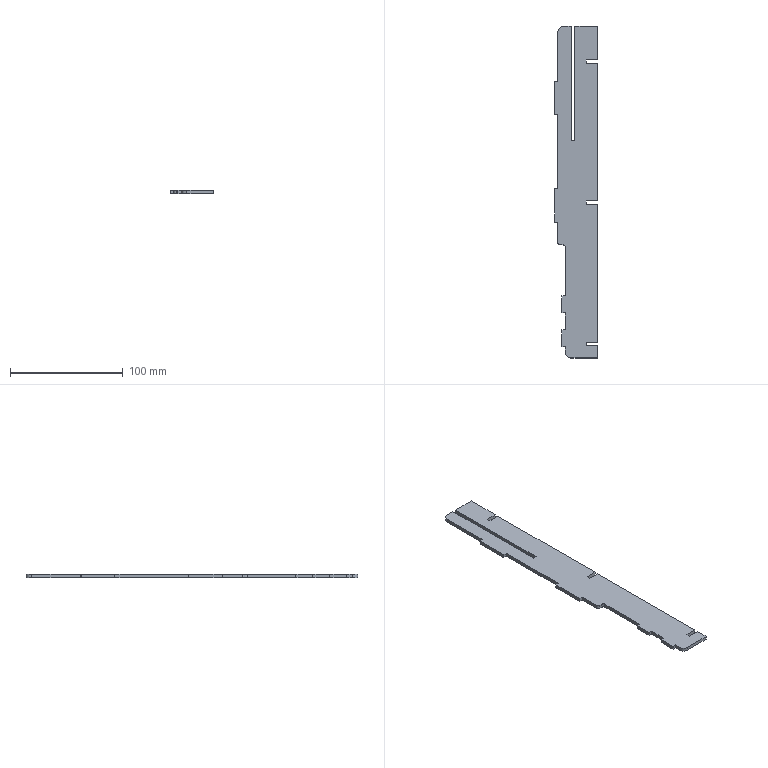Part | SolidWorks | features FlatPattern 1, SMBaseFlange 1, SheetMetal 1 | 1 solid | 46 faces | box 38 x 294.081 x 3.2 mm | volume 30340 mm3 | plane 40 | cylinder 6 | commonest cylinder face diameters 1 x2 4 x2 10 x2
STEP:
#1=CARTESIAN_POINT('',(-378.4,-209.357,0.));
#2=VERTEX_POINT('',#1);
#3=CARTESIAN_POINT('',(-378.4,-198.476,0.));
#4=VERTEX_POINT('',#3);
#5=CARTESIAN_POINT('',(-378.4,-198.476,0.));
#6=DIRECTION('',(-0.000000011,1.,0.));
#7=VECTOR('',#6,1000.);
#8=LINE('',#5,#7);
#9=EDGE_CURVE('',#2,#4,#8,.T.);
#10=ORIENTED_EDGE('',*,*,#9,.F.);
#11=CARTESIAN_POINT('',(-378.4,-209.357,-3.2));
#12=VERTEX_POINT('',#11);
#13=CARTESIAN_POINT('',(-378.4,-209.357,-3.2));
#14=DIRECTION('',(0.,0.,1.));
#15=VECTOR('',#14,1000.);
#16=LINE('',#13,#15);
#17=EDGE_CURVE('',#12,#2,#16,.T.);
#18=ORIENTED_EDGE('',*,*,#17,.F.);
#19=CARTESIAN_POINT('',(-378.4,-198.476,-3.2));
#20=VERTEX_POINT('',#19);
#21=CARTESIAN_POINT('',(-378.4,-198.476,-3.2));
#22=DIRECTION('',(-0.000000011,1.,0.));
#23=VECTOR('',#22,1000.);
#24=LINE('',#21,#23);
#25=EDGE_CURVE('',#12,#20,#24,.T.);
#26=ORIENTED_EDGE('',*,*,#25,.T.);
#27=CARTESIAN_POINT('',(-378.4,-198.476,-3.2));
#28=DIRECTION('',(0.,0.,1.));
#29=VECTOR('',#28,1000.);
#30=LINE('',#27,#29);
#31=EDGE_CURVE('',#20,#4,#30,.T.);
#32=ORIENTED_EDGE('',*,*,#31,.T.);
#33=EDGE_LOOP('',(#10,#18,#26,#32));
#34=FACE_OUTER_BOUND('',#33,.T.);
#35=CARTESIAN_POINT('',(-378.4,-198.476,-3.2));
#36=DIRECTION('',(1.,0.000000011,0.));
#37=DIRECTION('',(-0.000000011,1.,0.));
#38=AXIS2_PLACEMENT_3D('',#35,#36,#37);
#39=PLANE('',#38);
#40=ADVANCED_FACE('',(#34),#39,.T.);
#41=CARTESIAN_POINT('',(-401.9,-209.357,0.));
#42=VERTEX_POINT('',#41);
#43=CARTESIAN_POINT('',(-401.9,-209.357,0.));
#44=DIRECTION('',(1.,0.,0.));
#45=VECTOR('',#44,1000.);
#46=LINE('',#43,#45);
#47=EDGE_CURVE('',#42,#2,#46,.T.);
#48=ORIENTED_EDGE('',*,*,#47,.F.);
#49=CARTESIAN_POINT('',(-401.9,-209.357,-3.2));
#50=VERTEX_POINT('',#49);
#51=CARTESIAN_POINT('',(-401.9,-209.357,-3.2));
#52=DIRECTION('',(0.,0.,1.));
#53=VECTOR('',#52,1000.);
#54=LINE('',#51,#53);
#55=EDGE_CURVE('',#50,#42,#54,.T.);
#56=ORIENTED_EDGE('',*,*,#55,.F.);
#57=CARTESIAN_POINT('',(-401.9,-209.357,-3.2));
#58=DIRECTION('',(1.,0.,0.));
#59=VECTOR('',#58,1000.);
#60=LINE('',#57,#59);
#61=EDGE_CURVE('',#50,#12,#60,.T.);
#62=ORIENTED_EDGE('',*,*,#61,.T.);
#63=ORIENTED_EDGE('',*,*,#17,.T.);
#64=EDGE_LOOP('',(#48,#56,#62,#63));
#65=FACE_OUTER_BOUND('',#64,.T.);
#66=CARTESIAN_POINT('',(-401.9,-209.357,-3.2));
#67=DIRECTION('',(0.,-1.,0.));
#68=DIRECTION('',(0.,0.,-1.));
#69=AXIS2_PLACEMENT_3D('',#66,#67,#68);
#70=PLANE('',#69);
#71=ADVANCED_FACE('',(#65),#70,.T.);
#72=CARTESIAN_POINT('',(-406.9,-204.357,0.));
#73=VERTEX_POINT('',#72);
#74=CARTESIAN_POINT('',(-401.9,-204.357,0.));
#75=DIRECTION('',(0.,0.,1.));
#76=DIRECTION('',(-1.,0.,0.));
#77=AXIS2_PLACEMENT_3D('',#74,#75,#76);
#78=CIRCLE('',#77,5.);
#79=EDGE_CURVE('',#73,#42,#78,.T.);
#80=ORIENTED_EDGE('',*,*,#79,.F.);
#81=CARTESIAN_POINT('',(-406.9,-204.357,-3.2));
#82=VERTEX_POINT('',#81);
#83=CARTESIAN_POINT('',(-406.9,-204.357,-3.2));
#84=DIRECTION('',(0.,0.,1.));
#85=VECTOR('',#84,1000.);
#86=LINE('',#83,#85);
#87=EDGE_CURVE('',#82,#73,#86,.T.);
#88=ORIENTED_EDGE('',*,*,#87,.F.);
#89=CARTESIAN_POINT('',(-401.9,-204.357,-3.2));
#90=DIRECTION('',(0.,0.,1.));
#91=DIRECTION('',(-1.,0.,0.));
#92=AXIS2_PLACEMENT_3D('',#89,#90,#91);
#93=CIRCLE('',#92,5.);
#94=EDGE_CURVE('',#82,#50,#93,.T.);
#95=ORIENTED_EDGE('',*,*,#94,.T.);
#96=ORIENTED_EDGE('',*,*,#55,.T.);
#97=EDGE_LOOP('',(#80,#88,#95,#96));
#98=FACE_OUTER_BOUND('',#97,.T.);
#99=CARTESIAN_POINT('',(-401.9,-204.357,-3.2));
#100=DIRECTION('',(0.,0.,1.));
#101=DIRECTION('',(1.,0.,0.));
#102=AXIS2_PLACEMENT_3D('',#99,#100,#101);
#103=CYLINDRICAL_SURFACE('',#102,5.);
#104=ADVANCED_FACE('',(#98),#103,.T.);
#105=CARTESIAN_POINT('',(-406.9,-199.357,0.));
#106=VERTEX_POINT('',#105);
#107=CARTESIAN_POINT('',(-406.9,-199.357,0.));
#108=DIRECTION('',(0.,-1.,0.));
#109=VECTOR('',#108,1000.);
#110=LINE('',#107,#109);
#111=EDGE_CURVE('',#106,#73,#110,.T.);
#112=ORIENTED_EDGE('',*,*,#111,.F.);
#113=CARTESIAN_POINT('',(-406.9,-199.357,-3.2));
#114=VERTEX_POINT('',#113);
#115=CARTESIAN_POINT('',(-406.9,-199.357,-3.2));
#116=DIRECTION('',(0.,0.,1.));
#117=VECTOR('',#116,1000.);
#118=LINE('',#115,#117);
#119=EDGE_CURVE('',#114,#106,#118,.T.);
#120=ORIENTED_EDGE('',*,*,#119,.F.);
#121=CARTESIAN_POINT('',(-406.9,-199.357,-3.2));
#122=DIRECTION('',(0.,-1.,0.));
#123=VECTOR('',#122,1000.);
#124=LINE('',#121,#123);
#125=EDGE_CURVE('',#114,#82,#124,.T.);
#126=ORIENTED_EDGE('',*,*,#125,.T.);
#127=ORIENTED_EDGE('',*,*,#87,.T.);
#128=EDGE_LOOP('',(#112,#120,#126,#127));
#129=FACE_OUTER_BOUND('',#128,.T.);
#130=CARTESIAN_POINT('',(-406.9,-199.357,-3.2));
#131=DIRECTION('',(-1.,0.,0.));
#132=DIRECTION('',(0.,0.,1.));
#133=AXIS2_PLACEMENT_3D('',#130,#131,#132);
#134=PLANE('',#133);
#135=ADVANCED_FACE('',(#129),#134,.T.);
#136=CARTESIAN_POINT('',(-409.9,-199.357,0.));
#137=VERTEX_POINT('',#136);
#138=CARTESIAN_POINT('',(-409.9,-199.357,0.));
#139=DIRECTION('',(1.,0.,0.));
#140=VECTOR('',#139,1000.);
#141=LINE('',#138,#140);
#142=EDGE_CURVE('',#137,#106,#141,.T.);
#143=ORIENTED_EDGE('',*,*,#142,.F.);
#144=CARTESIAN_POINT('',(-409.9,-199.357,-3.2));
#145=VERTEX_POINT('',#144);
#146=CARTESIAN_POINT('',(-409.9,-199.357,-3.2));
#147=DIRECTION('',(0.,0.,1.));
#148=VECTOR('',#147,1000.);
#149=LINE('',#146,#148);
#150=EDGE_CURVE('',#145,#137,#149,.T.);
#151=ORIENTED_EDGE('',*,*,#150,.F.);
#152=CARTESIAN_POINT('',(-409.9,-199.357,-3.2));
#153=DIRECTION('',(1.,0.,0.));
#154=VECTOR('',#153,1000.);
#155=LINE('',#152,#154);
#156=EDGE_CURVE('',#145,#114,#155,.T.);
#157=ORIENTED_EDGE('',*,*,#156,.T.);
#158=ORIENTED_EDGE('',*,*,#119,.T.);
#159=EDGE_LOOP('',(#143,#151,#157,#158));
#160=FACE_OUTER_BOUND('',#159,.T.);
#161=CARTESIAN_POINT('',(-409.9,-199.357,-3.2));
#162=DIRECTION('',(0.,-1.,0.));
#163=DIRECTION('',(0.,0.,-1.));
#164=AXIS2_PLACEMENT_3D('',#161,#162,#163);
#165=PLANE('',#164);
#166=ADVANCED_FACE('',(#160),#165,.T.);
#167=CARTESIAN_POINT('',(-409.9,-184.357,0.));
#168=VERTEX_POINT('',#167);
#169=CARTESIAN_POINT('',(-409.9,-184.357,0.));
#170=DIRECTION('',(0.,-1.,0.));
#171=VECTOR('',#170,1000.);
#172=LINE('',#169,#171);
#173=EDGE_CURVE('',#168,#137,#172,.T.);
#174=ORIENTED_EDGE('',*,*,#173,.F.);
#175=CARTESIAN_POINT('',(-409.9,-184.357,-3.2));
#176=VERTEX_POINT('',#175);
#177=CARTESIAN_POINT('',(-409.9,-184.357,-3.2));
#178=DIRECTION('',(0.,0.,1.));
#179=VECTOR('',#178,1000.);
#180=LINE('',#177,#179);
#181=EDGE_CURVE('',#176,#168,#180,.T.);
#182=ORIENTED_EDGE('',*,*,#181,.F.);
#183=CARTESIAN_POINT('',(-409.9,-184.357,-3.2));
#184=DIRECTION('',(0.,-1.,0.));
#185=VECTOR('',#184,1000.);
#186=LINE('',#183,#185);
#187=EDGE_CURVE('',#176,#145,#186,.T.);
#188=ORIENTED_EDGE('',*,*,#187,.T.);
#189=ORIENTED_EDGE('',*,*,#150,.T.);
#190=EDGE_LOOP('',(#174,#182,#188,#189));
#191=FACE_OUTER_BOUND('',#190,.T.);
#192=CARTESIAN_POINT('',(-409.9,-184.357,-3.2));
#193=DIRECTION('',(-1.,0.,0.));
#194=DIRECTION('',(0.,0.,1.));
#195=AXIS2_PLACEMENT_3D('',#192,#193,#194);
#196=PLANE('',#195);
#197=ADVANCED_FACE('',(#191),#196,.T.);
#198=CARTESIAN_POINT('',(-406.9,-184.357,0.));
#199=VERTEX_POINT('',#198);
#200=CARTESIAN_POINT('',(-406.9,-184.357,0.));
#201=DIRECTION('',(-1.,0.,0.));
#202=VECTOR('',#201,1000.);
#203=LINE('',#200,#202);
#204=EDGE_CURVE('',#199,#168,#203,.T.);
#205=ORIENTED_EDGE('',*,*,#204,.F.);
#206=CARTESIAN_POINT('',(-406.9,-184.357,-3.2));
#207=VERTEX_POINT('',#206);
#208=CARTESIAN_POINT('',(-406.9,-184.357,-3.2));
#209=DIRECTION('',(0.,0.,1.));
#210=VECTOR('',#209,1000.);
#211=LINE('',#208,#210);
#212=EDGE_CURVE('',#207,#199,#211,.T.);
#213=ORIENTED_EDGE('',*,*,#212,.F.);
#214=CARTESIAN_POINT('',(-406.9,-184.357,-3.2));
#215=DIRECTION('',(-1.,0.,0.));
#216=VECTOR('',#215,1000.);
#217=LINE('',#214,#216);
#218=EDGE_CURVE('',#207,#176,#217,.T.);
#219=ORIENTED_EDGE('',*,*,#218,.T.);
#220=ORIENTED_EDGE('',*,*,#181,.T.);
#221=EDGE_LOOP('',(#205,#213,#219,#220));
#222=FACE_OUTER_BOUND('',#221,.T.);
#223=CARTESIAN_POINT('',(-406.9,-184.357,-3.2));
#224=DIRECTION('',(0.,1.,0.));
#225=DIRECTION('',(-1.,0.,0.));
#226=AXIS2_PLACEMENT_3D('',#223,#224,#225);
#227=PLANE('',#226);
#228=ADVANCED_FACE('',(#222),#227,.T.);
#229=CARTESIAN_POINT('',(-406.9,-169.357,0.));
#230=VERTEX_POINT('',#229);
#231=CARTESIAN_POINT('',(-406.9,-169.357,0.));
#232=DIRECTION('',(0.,-1.,0.));
#233=VECTOR('',#232,1000.);
#234=LINE('',#231,#233);
#235=EDGE_CURVE('',#230,#199,#234,.T.);
#236=ORIENTED_EDGE('',*,*,#235,.F.);
#237=CARTESIAN_POINT('',(-406.9,-169.357,-3.2));
#238=VERTEX_POINT('',#237);
#239=CARTESIAN_POINT('',(-406.9,-169.357,-3.2));
#240=DIRECTION('',(0.,0.,1.));
#241=VECTOR('',#240,1000.);
#242=LINE('',#239,#241);
#243=EDGE_CURVE('',#238,#230,#242,.T.);
#244=ORIENTED_EDGE('',*,*,#243,.F.);
#245=CARTESIAN_POINT('',(-406.9,-169.357,-3.2));
#246=DIRECTION('',(0.,-1.,0.));
#247=VECTOR('',#246,1000.);
#248=LINE('',#245,#247);
#249=EDGE_CURVE('',#238,#207,#248,.T.);
#250=ORIENTED_EDGE('',*,*,#249,.T.);
#251=ORIENTED_EDGE('',*,*,#212,.T.);
#252=EDGE_LOOP('',(#236,#244,#250,#251));
#253=FACE_OUTER_BOUND('',#252,.T.);
#254=CARTESIAN_POINT('',(-406.9,-169.357,-3.2));
#255=DIRECTION('',(-1.,0.,0.));
#256=DIRECTION('',(0.,0.,1.));
#257=AXIS2_PLACEMENT_3D('',#254,#255,#256);
#258=PLANE('',#257);
#259=ADVANCED_FACE('',(#253),#258,.T.);
#260=CARTESIAN_POINT('',(-409.9,-169.357,0.));
#261=VERTEX_POINT('',#260);
#262=CARTESIAN_POINT('',(-409.9,-169.357,0.));
#263=DIRECTION('',(1.,0.,0.));
#264=VECTOR('',#263,1000.);
#265=LINE('',#262,#264);
#266=EDGE_CURVE('',#261,#230,#265,.T.);
#267=ORIENTED_EDGE('',*,*,#266,.F.);
#268=CARTESIAN_POINT('',(-409.9,-169.357,-3.2));
#269=VERTEX_POINT('',#268);
#270=CARTESIAN_POINT('',(-409.9,-169.357,-3.2));
#271=DIRECTION('',(0.,0.,1.));
#272=VECTOR('',#271,1000.);
#273=LINE('',#270,#272);
#274=EDGE_CURVE('',#269,#261,#273,.T.);
#275=ORIENTED_EDGE('',*,*,#274,.F.);
#276=CARTESIAN_POINT('',(-409.9,-169.357,-3.2));
#277=DIRECTION('',(1.,0.,0.));
#278=VECTOR('',#277,1000.);
#279=LINE('',#276,#278);
#280=EDGE_CURVE('',#269,#238,#279,.T.);
#281=ORIENTED_EDGE('',*,*,#280,.T.);
#282=ORIENTED_EDGE('',*,*,#243,.T.);
#283=EDGE_LOOP('',(#267,#275,#281,#282));
#284=FACE_OUTER_BOUND('',#283,.T.);
#285=CARTESIAN_POINT('',(-409.9,-169.357,-3.2));
#286=DIRECTION('',(0.,-1.,0.));
#287=DIRECTION('',(0.,0.,-1.));
#288=AXIS2_PLACEMENT_3D('',#285,#286,#287);
#289=PLANE('',#288);
#290=ADVANCED_FACE('',(#284),#289,.T.);
#291=CARTESIAN_POINT('',(-409.9,-154.357,0.));
#292=VERTEX_POINT('',#291);
#293=CARTESIAN_POINT('',(-409.9,-154.357,0.));
#294=DIRECTION('',(0.,-1.,0.));
#295=VECTOR('',#294,1000.);
#296=LINE('',#293,#295);
#297=EDGE_CURVE('',#292,#261,#296,.T.);
#298=ORIENTED_EDGE('',*,*,#297,.F.);
#299=CARTESIAN_POINT('',(-409.9,-154.357,-3.2));
#300=VERTEX_POINT('',#299);
#301=CARTESIAN_POINT('',(-409.9,-154.357,-3.2));
#302=DIRECTION('',(0.,0.,1.));
#303=VECTOR('',#302,1000.);
#304=LINE('',#301,#303);
#305=EDGE_CURVE('',#300,#292,#304,.T.);
#306=ORIENTED_EDGE('',*,*,#305,.F.);
#307=CARTESIAN_POINT('',(-409.9,-154.357,-3.2));
#308=DIRECTION('',(0.,-1.,0.));
#309=VECTOR('',#308,1000.);
#310=LINE('',#307,#309);
#311=EDGE_CURVE('',#300,#269,#310,.T.);
#312=ORIENTED_EDGE('',*,*,#311,.T.);
#313=ORIENTED_EDGE('',*,*,#274,.T.);
#314=EDGE_LOOP('',(#298,#306,#312,#313));
#315=FACE_OUTER_BOUND('',#314,.T.);
#316=CARTESIAN_POINT('',(-409.9,-154.357,-3.2));
#317=DIRECTION('',(-1.,0.,0.));
#318=DIRECTION('',(0.,0.,1.));
#319=AXIS2_PLACEMENT_3D('',#316,#317,#318);
#320=PLANE('',#319);
#321=ADVANCED_FACE('',(#315),#320,.T.);
#322=CARTESIAN_POINT('',(-406.9,-154.357,0.));
#323=VERTEX_POINT('',#322);
#324=CARTESIAN_POINT('',(-406.9,-154.357,0.));
#325=DIRECTION('',(-1.,0.,0.));
#326=VECTOR('',#325,1000.);
#327=LINE('',#324,#326);
#328=EDGE_CURVE('',#323,#292,#327,.T.);
#329=ORIENTED_EDGE('',*,*,#328,.F.);
#330=CARTESIAN_POINT('',(-406.9,-154.357,-3.2));
#331=VERTEX_POINT('',#330);
#332=CARTESIAN_POINT('',(-406.9,-154.357,-3.2));
#333=DIRECTION('',(0.,0.,1.));
#334=VECTOR('',#333,1000.);
#335=LINE('',#332,#334);
#336=EDGE_CURVE('',#331,#323,#335,.T.);
#337=ORIENTED_EDGE('',*,*,#336,.F.);
#338=CARTESIAN_POINT('',(-406.9,-154.357,-3.2));
#339=DIRECTION('',(-1.,0.,0.));
#340=VECTOR('',#339,1000.);
#341=LINE('',#338,#340);
#342=EDGE_CURVE('',#331,#300,#341,.T.);
#343=ORIENTED_EDGE('',*,*,#342,.T.);
#344=ORIENTED_EDGE('',*,*,#305,.T.);
#345=EDGE_LOOP('',(#329,#337,#343,#344));
#346=FACE_OUTER_BOUND('',#345,.T.);
#347=CARTESIAN_POINT('',(-406.9,-154.357,-3.2));
#348=DIRECTION('',(0.,1.,0.));
#349=DIRECTION('',(0.,0.,1.));
#350=AXIS2_PLACEMENT_3D('',#347,#348,#349);
#351=PLANE('',#350);
#352=ADVANCED_FACE('',(#346),#351,.T.);
#353=CARTESIAN_POINT('',(-406.9,-111.086,0.));
#354=VERTEX_POINT('',#353);
#355=CARTESIAN_POINT('',(-406.9,-111.086,0.));
#356=DIRECTION('',(0.,-1.,0.));
#357=VECTOR('',#356,1000.);
#358=LINE('',#355,#357);
#359=EDGE_CURVE('',#354,#323,#358,.T.);
#360=ORIENTED_EDGE('',*,*,#359,.F.);
#361=CARTESIAN_POINT('',(-406.9,-111.086,-3.2));
#362=VERTEX_POINT('',#361);
#363=CARTESIAN_POINT('',(-406.9,-111.086,-3.2));
#364=DIRECTION('',(0.,0.,1.));
#365=VECTOR('',#364,1000.);
#366=LINE('',#363,#365);
#367=EDGE_CURVE('',#362,#354,#366,.T.);
#368=ORIENTED_EDGE('',*,*,#367,.F.);
#369=CARTESIAN_POINT('',(-406.9,-111.086,-3.2));
#370=DIRECTION('',(0.,-1.,0.));
#371=VECTOR('',#370,1000.);
#372=LINE('',#369,#371);
#373=EDGE_CURVE('',#362,#331,#372,.T.);
#374=ORIENTED_EDGE('',*,*,#373,.T.);
#375=ORIENTED_EDGE('',*,*,#336,.T.);
#376=EDGE_LOOP('',(#360,#368,#374,#375));
#377=FACE_OUTER_BOUND('',#376,.T.);
#378=CARTESIAN_POINT('',(-406.9,-111.086,-3.2));
#379=DIRECTION('',(-1.,0.,0.));
#380=DIRECTION('',(0.,0.,1.));
#381=AXIS2_PLACEMENT_3D('',#378,#379,#380);
#382=PLANE('',#381);
#383=ADVANCED_FACE('',(#377),#382,.T.);
#384=CARTESIAN_POINT('',(-408.9,-109.086,0.));
#385=VERTEX_POINT('',#384);
#386=CARTESIAN_POINT('',(-408.9,-111.086,0.));
#387=DIRECTION('',(0.,0.,-1.));
#388=DIRECTION('',(-1.,0.,0.));
#389=AXIS2_PLACEMENT_3D('',#386,#387,#388);
#390=CIRCLE('',#389,2.);
#391=EDGE_CURVE('',#385,#354,#390,.T.);
#392=ORIENTED_EDGE('',*,*,#391,.F.);
#393=CARTESIAN_POINT('',(-408.9,-109.086,-3.2));
#394=VERTEX_POINT('',#393);
#395=CARTESIAN_POINT('',(-408.9,-109.086,-3.2));
#396=DIRECTION('',(0.,0.,1.));
#397=VECTOR('',#396,1000.);
#398=LINE('',#395,#397);
#399=EDGE_CURVE('',#394,#385,#398,.T.);
#400=ORIENTED_EDGE('',*,*,#399,.F.);
#401=CARTESIAN_POINT('',(-408.9,-111.086,-3.2));
#402=DIRECTION('',(0.,0.,-1.));
#403=DIRECTION('',(-1.,0.,0.));
#404=AXIS2_PLACEMENT_3D('',#401,#402,#403);
#405=CIRCLE('',#404,2.);
#406=EDGE_CURVE('',#394,#362,#405,.T.);
#407=ORIENTED_EDGE('',*,*,#406,.T.);
#408=ORIENTED_EDGE('',*,*,#367,.T.);
#409=EDGE_LOOP('',(#392,#400,#407,#408));
#410=FACE_OUTER_BOUND('',#409,.T.);
#411=CARTESIAN_POINT('',(-408.9,-111.086,-3.2));
#412=DIRECTION('',(0.,0.,1.));
#413=DIRECTION('',(1.,0.,0.));
#414=AXIS2_PLACEMENT_3D('',#411,#412,#413);
#415=CYLINDRICAL_SURFACE('',#414,2.);
#416=ADVANCED_FACE('',(#410),#415,.F.);
#417=CARTESIAN_POINT('',(-411.4,-109.086,0.));
#418=VERTEX_POINT('',#417);
#419=CARTESIAN_POINT('',(-408.9,-109.086,0.));
#420=DIRECTION('',(1.,0.,0.));
#421=VECTOR('',#420,1000.);
#422=LINE('',#419,#421);
#423=EDGE_CURVE('',#418,#385,#422,.T.);
#424=ORIENTED_EDGE('',*,*,#423,.F.);
#425=CARTESIAN_POINT('',(-411.4,-109.086,-3.2));
#426=VERTEX_POINT('',#425);
#427=CARTESIAN_POINT('',(-411.4,-109.086,-3.2));
#428=DIRECTION('',(0.,0.,1.));
#429=VECTOR('',#428,1000.);
#430=LINE('',#427,#429);
#431=EDGE_CURVE('',#426,#418,#430,.T.);
#432=ORIENTED_EDGE('',*,*,#431,.F.);
#433=CARTESIAN_POINT('',(-408.9,-109.086,-3.2));
#434=DIRECTION('',(1.,0.,0.));
#435=VECTOR('',#434,1000.);
#436=LINE('',#433,#435);
#437=EDGE_CURVE('',#426,#394,#436,.T.);
#438=ORIENTED_EDGE('',*,*,#437,.T.);
#439=ORIENTED_EDGE('',*,*,#399,.T.);
#440=EDGE_LOOP('',(#424,#432,#438,#439));
#441=FACE_OUTER_BOUND('',#440,.T.);
#442=CARTESIAN_POINT('',(-408.9,-109.086,-3.2));
#443=DIRECTION('',(0.,-1.,0.));
#444=DIRECTION('',(0.,0.,-1.));
#445=AXIS2_PLACEMENT_3D('',#442,#443,#444);
#446=PLANE('',#445);
#447=ADVANCED_FACE('',(#441),#446,.T.);
#448=CARTESIAN_POINT('',(-413.4,-107.086,0.));
#449=VERTEX_POINT('',#448);
#450=CARTESIAN_POINT('',(-411.4,-107.086,0.));
#451=DIRECTION('',(0.,0.,1.));
#452=DIRECTION('',(-1.,0.,0.));
#453=AXIS2_PLACEMENT_3D('',#450,#451,#452);
#454=CIRCLE('',#453,2.);
#455=EDGE_CURVE('',#449,#418,#454,.T.);
#456=ORIENTED_EDGE('',*,*,#455,.F.);
#457=CARTESIAN_POINT('',(-413.4,-107.086,-3.2));
#458=VERTEX_POINT('',#457);
#459=CARTESIAN_POINT('',(-413.4,-107.086,-3.2));
#460=DIRECTION('',(0.,0.,1.));
#461=VECTOR('',#460,1000.);
#462=LINE('',#459,#461);
#463=EDGE_CURVE('',#458,#449,#462,.T.);
#464=ORIENTED_EDGE('',*,*,#463,.F.);
#465=CARTESIAN_POINT('',(-411.4,-107.086,-3.2));
#466=DIRECTION('',(0.,0.,1.));
#467=DIRECTION('',(-1.,0.,0.));
#468=AXIS2_PLACEMENT_3D('',#465,#466,#467);
#469=CIRCLE('',#468,2.);
#470=EDGE_CURVE('',#458,#426,#469,.T.);
#471=ORIENTED_EDGE('',*,*,#470,.T.);
#472=ORIENTED_EDGE('',*,*,#431,.T.);
#473=EDGE_LOOP('',(#456,#464,#471,#472));
#474=FACE_OUTER_BOUND('',#473,.T.);
#475=CARTESIAN_POINT('',(-411.4,-107.086,-3.2));
#476=DIRECTION('',(0.,0.,1.));
#477=DIRECTION('',(1.,0.,0.));
#478=AXIS2_PLACEMENT_3D('',#475,#476,#477);
#479=CYLINDRICAL_SURFACE('',#478,2.);
#480=ADVANCED_FACE('',(#474),#479,.T.);
#481=CARTESIAN_POINT('',(-413.4,-89.086,0.));
#482=VERTEX_POINT('',#481);
#483=CARTESIAN_POINT('',(-413.4,-89.086,0.));
#484=DIRECTION('',(0.,-1.,0.));
#485=VECTOR('',#484,1000.);
#486=LINE('',#483,#485);
#487=EDGE_CURVE('',#482,#449,#486,.T.);
#488=ORIENTED_EDGE('',*,*,#487,.F.);
#489=CARTESIAN_POINT('',(-413.4,-89.086,-3.2));
#490=VERTEX_POINT('',#489);
#491=CARTESIAN_POINT('',(-413.4,-89.086,-3.2));
#492=DIRECTION('',(0.,0.,1.));
#493=VECTOR('',#492,1000.);
#494=LINE('',#491,#493);
#495=EDGE_CURVE('',#490,#482,#494,.T.);
#496=ORIENTED_EDGE('',*,*,#495,.F.);
#497=CARTESIAN_POINT('',(-413.4,-89.086,-3.2));
#498=DIRECTION('',(0.,-1.,0.));
#499=VECTOR('',#498,1000.);
#500=LINE('',#497,#499);
#501=EDGE_CURVE('',#490,#458,#500,.T.);
#502=ORIENTED_EDGE('',*,*,#501,.T.);
#503=ORIENTED_EDGE('',*,*,#463,.T.);
#504=EDGE_LOOP('',(#488,#496,#502,#503));
#505=FACE_OUTER_BOUND('',#504,.T.);
#506=CARTESIAN_POINT('',(-413.4,-89.086,-3.2));
#507=DIRECTION('',(-1.,0.,0.));
#508=DIRECTION('',(0.,0.,1.));
#509=AXIS2_PLACEMENT_3D('',#506,#507,#508);
#510=PLANE('',#509);
#511=ADVANCED_FACE('',(#505),#510,.T.);
#512=CARTESIAN_POINT('',(-416.4,-89.086,0.));
#513=VERTEX_POINT('',#512);
#514=CARTESIAN_POINT('',(-416.4,-89.086,0.));
#515=DIRECTION('',(1.,0.,0.));
#516=VECTOR('',#515,1000.);
#517=LINE('',#514,#516);
#518=EDGE_CURVE('',#513,#482,#517,.T.);
#519=ORIENTED_EDGE('',*,*,#518,.F.);
#520=CARTESIAN_POINT('',(-416.4,-89.086,-3.2));
#521=VERTEX_POINT('',#520);
#522=CARTESIAN_POINT('',(-416.4,-89.086,-3.2));
#523=DIRECTION('',(0.,0.,1.));
#524=VECTOR('',#523,1000.);
#525=LINE('',#522,#524);
#526=EDGE_CURVE('',#521,#513,#525,.T.);
#527=ORIENTED_EDGE('',*,*,#526,.F.);
#528=CARTESIAN_POINT('',(-416.4,-89.086,-3.2));
#529=DIRECTION('',(1.,0.,0.));
#530=VECTOR('',#529,1000.);
#531=LINE('',#528,#530);
#532=EDGE_CURVE('',#521,#490,#531,.T.);
#533=ORIENTED_EDGE('',*,*,#532,.T.);
#534=ORIENTED_EDGE('',*,*,#495,.T.);
#535=EDGE_LOOP('',(#519,#527,#533,#534));
#536=FACE_OUTER_BOUND('',#535,.T.);
#537=CARTESIAN_POINT('',(-416.4,-89.086,-3.2));
#538=DIRECTION('',(0.,-1.,0.));
#539=DIRECTION('',(0.,0.,-1.));
#540=AXIS2_PLACEMENT_3D('',#537,#538,#539);
#541=PLANE('',#540);
#542=ADVANCED_FACE('',(#536),#541,.T.);
#543=CARTESIAN_POINT('',(-416.4,-59.086,0.));
#544=VERTEX_POINT('',#543);
#545=CARTESIAN_POINT('',(-416.4,-59.086,0.));
#546=DIRECTION('',(0.,-1.,0.));
#547=VECTOR('',#546,1000.);
#548=LINE('',#545,#547);
#549=EDGE_CURVE('',#544,#513,#548,.T.);
#550=ORIENTED_EDGE('',*,*,#549,.F.);
#551=CARTESIAN_POINT('',(-416.4,-59.086,-3.2));
#552=VERTEX_POINT('',#551);
#553=CARTESIAN_POINT('',(-416.4,-59.086,-3.2));
#554=DIRECTION('',(0.,0.,1.));
#555=VECTOR('',#554,1000.);
#556=LINE('',#553,#555);
#557=EDGE_CURVE('',#552,#544,#556,.T.);
#558=ORIENTED_EDGE('',*,*,#557,.F.);
#559=CARTESIAN_POINT('',(-416.4,-59.086,-3.2));
#560=DIRECTION('',(0.,-1.,0.));
#561=VECTOR('',#560,1000.);
#562=LINE('',#559,#561);
#563=EDGE_CURVE('',#552,#521,#562,.T.);
#564=ORIENTED_EDGE('',*,*,#563,.T.);
#565=ORIENTED_EDGE('',*,*,#526,.T.);
#566=EDGE_LOOP('',(#550,#558,#564,#565));
#567=FACE_OUTER_BOUND('',#566,.T.);
#568=CARTESIAN_POINT('',(-416.4,-59.086,-3.2));
#569=DIRECTION('',(-1.,0.,0.));
#570=DIRECTION('',(0.,0.,1.));
#571=AXIS2_PLACEMENT_3D('',#568,#569,#570);
#572=PLANE('',#571);
#573=ADVANCED_FACE('',(#567),#572,.T.);
#574=CARTESIAN_POINT('',(-413.4,-59.086,0.));
#575=VERTEX_POINT('',#574);
#576=CARTESIAN_POINT('',(-413.4,-59.086,0.));
#577=DIRECTION('',(-1.,0.,0.));
#578=VECTOR('',#577,1000.);
#579=LINE('',#576,#578);
#580=EDGE_CURVE('',#575,#544,#579,.T.);
#581=ORIENTED_EDGE('',*,*,#580,.F.);
#582=CARTESIAN_POINT('',(-413.4,-59.086,-3.2));
#583=VERTEX_POINT('',#582);
#584=CARTESIAN_POINT('',(-413.4,-59.086,-3.2));
#585=DIRECTION('',(0.,0.,1.));
#586=VECTOR('',#585,1000.);
#587=LINE('',#584,#586);
#588=EDGE_CURVE('',#583,#575,#587,.T.);
#589=ORIENTED_EDGE('',*,*,#588,.F.);
#590=CARTESIAN_POINT('',(-413.4,-59.086,-3.2));
#591=DIRECTION('',(-1.,0.,0.));
#592=VECTOR('',#591,1000.);
#593=LINE('',#590,#592);
#594=EDGE_CURVE('',#583,#552,#593,.T.);
#595=ORIENTED_EDGE('',*,*,#594,.T.);
#596=ORIENTED_EDGE('',*,*,#557,.T.);
#597=EDGE_LOOP('',(#581,#589,#595,#596));
#598=FACE_OUTER_BOUND('',#597,.T.);
#599=CARTESIAN_POINT('',(-413.4,-59.086,-3.2));
#600=DIRECTION('',(0.,1.,0.));
#601=DIRECTION('',(0.,0.,1.));
#602=AXIS2_PLACEMENT_3D('',#599,#600,#601);
#603=PLANE('',#602);
#604=ADVANCED_FACE('',(#598),#603,.T.);
#605=CARTESIAN_POINT('',(-413.4,5.914,0.));
#606=VERTEX_POINT('',#605);
#607=CARTESIAN_POINT('',(-413.4,5.914,0.));
#608=DIRECTION('',(0.,-1.,0.));
#609=VECTOR('',#608,1000.);
#610=LINE('',#607,#609);
#611=EDGE_CURVE('',#606,#575,#610,.T.);
#612=ORIENTED_EDGE('',*,*,#611,.F.);
#613=CARTESIAN_POINT('',(-413.4,5.914,-3.2));
#614=VERTEX_POINT('',#613);
#615=CARTESIAN_POINT('',(-413.4,5.914,-3.2));
#616=DIRECTION('',(0.,0.,1.));
#617=VECTOR('',#616,1000.);
#618=LINE('',#615,#617);
#619=EDGE_CURVE('',#614,#606,#618,.T.);
#620=ORIENTED_EDGE('',*,*,#619,.F.);
#621=CARTESIAN_POINT('',(-413.4,5.914,-3.2));
#622=DIRECTION('',(0.,-1.,0.));
#623=VECTOR('',#622,1000.);
#624=LINE('',#621,#623);
#625=EDGE_CURVE('',#614,#583,#624,.T.);
#626=ORIENTED_EDGE('',*,*,#625,.T.);
#627=ORIENTED_EDGE('',*,*,#588,.T.);
#628=EDGE_LOOP('',(#612,#620,#626,#627));
#629=FACE_OUTER_BOUND('',#628,.T.);
#630=CARTESIAN_POINT('',(-413.4,5.914,-3.2));
#631=DIRECTION('',(-1.,0.,0.));
#632=DIRECTION('',(0.,0.,1.));
#633=AXIS2_PLACEMENT_3D('',#630,#631,#632);
#634=PLANE('',#633);
#635=ADVANCED_FACE('',(#629),#634,.T.);
#636=CARTESIAN_POINT('',(-416.4,5.914,0.));
#637=VERTEX_POINT('',#636);
#638=CARTESIAN_POINT('',(-416.4,5.914,0.));
#639=DIRECTION('',(1.,0.,0.));
#640=VECTOR('',#639,1000.);
#641=LINE('',#638,#640);
#642=EDGE_CURVE('',#637,#606,#641,.T.);
#643=ORIENTED_EDGE('',*,*,#642,.F.);
#644=CARTESIAN_POINT('',(-416.4,5.914,-3.2));
#645=VERTEX_POINT('',#644);
#646=CARTESIAN_POINT('',(-416.4,5.914,-3.2));
#647=DIRECTION('',(0.,0.,1.));
#648=VECTOR('',#647,1000.);
#649=LINE('',#646,#648);
#650=EDGE_CURVE('',#645,#637,#649,.T.);
#651=ORIENTED_EDGE('',*,*,#650,.F.);
#652=CARTESIAN_POINT('',(-416.4,5.914,-3.2));
#653=DIRECTION('',(1.,0.,0.));
#654=VECTOR('',#653,1000.);
#655=LINE('',#652,#654);
#656=EDGE_CURVE('',#645,#614,#655,.T.);
#657=ORIENTED_EDGE('',*,*,#656,.T.);
#658=ORIENTED_EDGE('',*,*,#619,.T.);
#659=EDGE_LOOP('',(#643,#651,#657,#658));
#660=FACE_OUTER_BOUND('',#659,.T.);
#661=CARTESIAN_POINT('',(-416.4,5.914,-3.2));
#662=DIRECTION('',(0.,-1.,0.));
#663=DIRECTION('',(0.,0.,-1.));
#664=AXIS2_PLACEMENT_3D('',#661,#662,#663);
#665=PLANE('',#664);
#666=ADVANCED_FACE('',(#660),#665,.T.);
#667=CARTESIAN_POINT('',(-416.4,35.414,0.));
#668=VERTEX_POINT('',#667);
#669=CARTESIAN_POINT('',(-416.4,35.414,0.));
#670=DIRECTION('',(0.,-1.,0.));
#671=VECTOR('',#670,1000.);
#672=LINE('',#669,#671);
#673=EDGE_CURVE('',#668,#637,#672,.T.);
#674=ORIENTED_EDGE('',*,*,#673,.F.);
#675=CARTESIAN_POINT('',(-416.4,35.414,-3.2));
#676=VERTEX_POINT('',#675);
#677=CARTESIAN_POINT('',(-416.4,35.414,-3.2));
#678=DIRECTION('',(0.,0.,1.));
#679=VECTOR('',#678,1000.);
#680=LINE('',#677,#679);
#681=EDGE_CURVE('',#676,#668,#680,.T.);
#682=ORIENTED_EDGE('',*,*,#681,.F.);
#683=CARTESIAN_POINT('',(-416.4,35.414,-3.2));
#684=DIRECTION('',(0.,-1.,0.));
#685=VECTOR('',#684,1000.);
#686=LINE('',#683,#685);
#687=EDGE_CURVE('',#676,#645,#686,.T.);
#688=ORIENTED_EDGE('',*,*,#687,.T.);
#689=ORIENTED_EDGE('',*,*,#650,.T.);
#690=EDGE_LOOP('',(#674,#682,#688,#689));
#691=FACE_OUTER_BOUND('',#690,.T.);
#692=CARTESIAN_POINT('',(-416.4,35.414,-3.2));
#693=DIRECTION('',(-1.,0.,0.));
#694=DIRECTION('',(0.,0.,1.));
#695=AXIS2_PLACEMENT_3D('',#692,#693,#694);
#696=PLANE('',#695);
#697=ADVANCED_FACE('',(#691),#696,.T.);
#698=CARTESIAN_POINT('',(-415.9,35.914,0.));
#699=VERTEX_POINT('',#698);
#700=CARTESIAN_POINT('',(-415.9,35.414,0.));
#701=DIRECTION('',(0.,0.,1.));
#702=DIRECTION('',(1.,0.,0.));
#703=AXIS2_PLACEMENT_3D('',#700,#701,#702);
#704=CIRCLE('',#703,0.5);
#705=EDGE_CURVE('',#699,#668,#704,.T.);
#706=ORIENTED_EDGE('',*,*,#705,.F.);
#707=CARTESIAN_POINT('',(-415.9,35.914,-3.2));
#708=VERTEX_POINT('',#707);
#709=CARTESIAN_POINT('',(-415.9,35.914,-3.2));
#710=DIRECTION('',(0.,0.,1.));
#711=VECTOR('',#710,1000.);
#712=LINE('',#709,#711);
#713=EDGE_CURVE('',#708,#699,#712,.T.);
#714=ORIENTED_EDGE('',*,*,#713,.F.);
#715=CARTESIAN_POINT('',(-415.9,35.414,-3.2));
#716=DIRECTION('',(0.,0.,1.));
#717=DIRECTION('',(1.,0.,0.));
#718=AXIS2_PLACEMENT_3D('',#715,#716,#717);
#719=CIRCLE('',#718,0.5);
#720=EDGE_CURVE('',#708,#676,#719,.T.);
#721=ORIENTED_EDGE('',*,*,#720,.T.);
#722=ORIENTED_EDGE('',*,*,#681,.T.);
#723=EDGE_LOOP('',(#706,#714,#721,#722));
#724=FACE_OUTER_BOUND('',#723,.T.);
#725=CARTESIAN_POINT('',(-415.9,35.414,-3.2));
#726=DIRECTION('',(0.,0.,1.));
#727=DIRECTION('',(1.,0.,0.));
#728=AXIS2_PLACEMENT_3D('',#725,#726,#727);
#729=CYLINDRICAL_SURFACE('',#728,0.5);
#730=ADVANCED_FACE('',(#724),#729,.T.);
#731=CARTESIAN_POINT('',(-413.9,35.914,0.));
#732=VERTEX_POINT('',#731);
#733=CARTESIAN_POINT('',(-413.9,35.914,0.));
#734=DIRECTION('',(-1.,0.,0.));
#735=VECTOR('',#734,1000.);
#736=LINE('',#733,#735);
#737=EDGE_CURVE('',#732,#699,#736,.T.);
#738=ORIENTED_EDGE('',*,*,#737,.F.);
#739=CARTESIAN_POINT('',(-413.9,35.914,-3.2));
#740=VERTEX_POINT('',#739);
#741=CARTESIAN_POINT('',(-413.9,35.914,-3.2));
#742=DIRECTION('',(0.,0.,1.));
#743=VECTOR('',#742,1000.);
#744=LINE('',#741,#743);
#745=EDGE_CURVE('',#740,#732,#744,.T.);
#746=ORIENTED_EDGE('',*,*,#745,.F.);
#747=CARTESIAN_POINT('',(-413.9,35.914,-3.2));
#748=DIRECTION('',(-1.,0.,0.));
#749=VECTOR('',#748,1000.);
#750=LINE('',#747,#749);
#751=EDGE_CURVE('',#740,#708,#750,.T.);
#752=ORIENTED_EDGE('',*,*,#751,.T.);
#753=ORIENTED_EDGE('',*,*,#713,.T.);
#754=EDGE_LOOP('',(#738,#746,#752,#753));
#755=FACE_OUTER_BOUND('',#754,.T.);
#756=CARTESIAN_POINT('',(-413.9,35.914,-3.2));
#757=DIRECTION('',(0.,1.,0.));
#758=DIRECTION('',(0.,0.,1.));
#759=AXIS2_PLACEMENT_3D('',#756,#757,#758);
#760=PLANE('',#759);
#761=ADVANCED_FACE('',(#755),#760,.T.);
#762=CARTESIAN_POINT('',(-413.4,36.414,0.));
#763=VERTEX_POINT('',#762);
#764=CARTESIAN_POINT('',(-413.9,36.414,0.));
#765=DIRECTION('',(0.,0.,-1.));
#766=DIRECTION('',(-1.,0.,0.));
#767=AXIS2_PLACEMENT_3D('',#764,#765,#766);
#768=CIRCLE('',#767,0.5);
#769=EDGE_CURVE('',#763,#732,#768,.T.);
#770=ORIENTED_EDGE('',*,*,#769,.F.);
#771=CARTESIAN_POINT('',(-413.4,36.414,-3.2));
#772=VERTEX_POINT('',#771);
#773=CARTESIAN_POINT('',(-413.4,36.414,-3.2));
#774=DIRECTION('',(0.,0.,1.));
#775=VECTOR('',#774,1000.);
#776=LINE('',#773,#775);
#777=EDGE_CURVE('',#772,#763,#776,.T.);
#778=ORIENTED_EDGE('',*,*,#777,.F.);
#779=CARTESIAN_POINT('',(-413.9,36.414,-3.2));
#780=DIRECTION('',(0.,0.,-1.));
#781=DIRECTION('',(-1.,0.,0.));
#782=AXIS2_PLACEMENT_3D('',#779,#780,#781);
#783=CIRCLE('',#782,0.5);
#784=EDGE_CURVE('',#772,#740,#783,.T.);
#785=ORIENTED_EDGE('',*,*,#784,.T.);
#786=ORIENTED_EDGE('',*,*,#745,.T.);
#787=EDGE_LOOP('',(#770,#778,#785,#786));
#788=FACE_OUTER_BOUND('',#787,.T.);
#789=CARTESIAN_POINT('',(-413.9,36.414,-3.2));
#790=DIRECTION('',(0.,0.,1.));
#791=DIRECTION('',(1.,0.,0.));
#792=AXIS2_PLACEMENT_3D('',#789,#790,#791);
#793=CYLINDRICAL_SURFACE('',#792,0.5);
#794=ADVANCED_FACE('',(#788),#793,.F.);
#795=CARTESIAN_POINT('',(-413.4,79.724,0.));
#796=VERTEX_POINT('',#795);
#797=CARTESIAN_POINT('',(-413.4,79.724,0.));
#798=DIRECTION('',(0.,-1.,0.));
#799=VECTOR('',#798,1000.);
#800=LINE('',#797,#799);
#801=EDGE_CURVE('',#796,#763,#800,.T.);
#802=ORIENTED_EDGE('',*,*,#801,.F.);
#803=CARTESIAN_POINT('',(-413.4,79.724,-3.2));
#804=VERTEX_POINT('',#803);
#805=CARTESIAN_POINT('',(-413.4,79.724,-3.2));
#806=DIRECTION('',(0.,0.,1.));
#807=VECTOR('',#806,1000.);
#808=LINE('',#805,#807);
#809=EDGE_CURVE('',#804,#796,#808,.T.);
#810=ORIENTED_EDGE('',*,*,#809,.F.);
#811=CARTESIAN_POINT('',(-413.4,79.724,-3.2));
#812=DIRECTION('',(0.,-1.,0.));
#813=VECTOR('',#812,1000.);
#814=LINE('',#811,#813);
#815=EDGE_CURVE('',#804,#772,#814,.T.);
#816=ORIENTED_EDGE('',*,*,#815,.T.);
#817=ORIENTED_EDGE('',*,*,#777,.T.);
#818=EDGE_LOOP('',(#802,#810,#816,#817));
#819=FACE_OUTER_BOUND('',#818,.T.);
#820=CARTESIAN_POINT('',(-413.4,79.724,-3.2));
#821=DIRECTION('',(-1.,0.,0.));
#822=DIRECTION('',(0.,0.,1.));
#823=AXIS2_PLACEMENT_3D('',#820,#821,#822);
#824=PLANE('',#823);
#825=ADVANCED_FACE('',(#819),#824,.T.);
#826=CARTESIAN_POINT('',(-408.4,84.724,0.));
#827=VERTEX_POINT('',#826);
#828=CARTESIAN_POINT('',(-408.4,79.724,0.));
#829=DIRECTION('',(0.,0.,1.));
#830=DIRECTION('',(1.,0.,0.));
#831=AXIS2_PLACEMENT_3D('',#828,#829,#830);
#832=CIRCLE('',#831,5.);
#833=EDGE_CURVE('',#827,#796,#832,.T.);
#834=ORIENTED_EDGE('',*,*,#833,.F.);
#835=CARTESIAN_POINT('',(-408.4,84.724,-3.2));
#836=VERTEX_POINT('',#835);
#837=CARTESIAN_POINT('',(-408.4,84.724,-3.2));
#838=DIRECTION('',(0.,0.,1.));
#839=VECTOR('',#838,1000.);
#840=LINE('',#837,#839);
#841=EDGE_CURVE('',#836,#827,#840,.T.);
#842=ORIENTED_EDGE('',*,*,#841,.F.);
#843=CARTESIAN_POINT('',(-408.4,79.724,-3.2));
#844=DIRECTION('',(0.,0.,1.));
#845=DIRECTION('',(1.,0.,0.));
#846=AXIS2_PLACEMENT_3D('',#843,#844,#845);
#847=CIRCLE('',#846,5.);
#848=EDGE_CURVE('',#836,#804,#847,.T.);
#849=ORIENTED_EDGE('',*,*,#848,.T.);
#850=ORIENTED_EDGE('',*,*,#809,.T.);
#851=EDGE_LOOP('',(#834,#842,#849,#850));
#852=FACE_OUTER_BOUND('',#851,.T.);
#853=CARTESIAN_POINT('',(-408.4,79.724,-3.2));
#854=DIRECTION('',(0.,0.,1.));
#855=DIRECTION('',(1.,0.,0.));
#856=AXIS2_PLACEMENT_3D('',#853,#854,#855);
#857=CYLINDRICAL_SURFACE('',#856,5.);
#858=ADVANCED_FACE('',(#852),#857,.T.);
#859=CARTESIAN_POINT('',(-401.6,84.724,0.));
#860=VERTEX_POINT('',#859);
#861=CARTESIAN_POINT('',(-401.6,84.724,0.));
#862=DIRECTION('',(-1.,-0.000000028,0.));
#863=VECTOR('',#862,1000.);
#864=LINE('',#861,#863);
#865=EDGE_CURVE('',#860,#827,#864,.T.);
#866=ORIENTED_EDGE('',*,*,#865,.F.);
#867=CARTESIAN_POINT('',(-401.6,84.724,-3.2));
#868=VERTEX_POINT('',#867);
#869=CARTESIAN_POINT('',(-401.6,84.724,-3.2));
#870=DIRECTION('',(0.,0.,1.));
#871=VECTOR('',#870,1000.);
#872=LINE('',#869,#871);
#873=EDGE_CURVE('',#868,#860,#872,.T.);
#874=ORIENTED_EDGE('',*,*,#873,.F.);
#875=CARTESIAN_POINT('',(-401.6,84.724,-3.2));
#876=DIRECTION('',(-1.,-0.000000028,0.));
#877=VECTOR('',#876,1000.);
#878=LINE('',#875,#877);
#879=EDGE_CURVE('',#868,#836,#878,.T.);
#880=ORIENTED_EDGE('',*,*,#879,.T.);
#881=ORIENTED_EDGE('',*,*,#841,.T.);
#882=EDGE_LOOP('',(#866,#874,#880,#881));
#883=FACE_OUTER_BOUND('',#882,.T.);
#884=CARTESIAN_POINT('',(-401.6,84.724,-3.2));
#885=DIRECTION('',(-0.000000028,1.,0.));
#886=DIRECTION('',(-1.,-0.000000028,0.));
#887=AXIS2_PLACEMENT_3D('',#884,#885,#886);
#888=PLANE('',#887);
#889=ADVANCED_FACE('',(#883),#888,.T.);
#890=CARTESIAN_POINT('',(-401.6,-16.276,0.));
#891=VERTEX_POINT('',#890);
#892=CARTESIAN_POINT('',(-401.6,84.724,0.));
#893=DIRECTION('',(0.,1.,0.));
#894=VECTOR('',#893,1000.);
#895=LINE('',#892,#894);
#896=EDGE_CURVE('',#891,#860,#895,.T.);
#897=ORIENTED_EDGE('',*,*,#896,.F.);
#898=CARTESIAN_POINT('',(-401.6,-16.276,-3.2));
#899=VERTEX_POINT('',#898);
#900=CARTESIAN_POINT('',(-401.6,-16.276,-3.2));
#901=DIRECTION('',(0.,0.,1.));
#902=VECTOR('',#901,1000.);
#903=LINE('',#900,#902);
#904=EDGE_CURVE('',#899,#891,#903,.T.);
#905=ORIENTED_EDGE('',*,*,#904,.F.);
#906=CARTESIAN_POINT('',(-401.6,84.724,-3.2));
#907=DIRECTION('',(0.,1.,0.));
#908=VECTOR('',#907,1000.);
#909=LINE('',#906,#908);
#910=EDGE_CURVE('',#899,#868,#909,.T.);
#911=ORIENTED_EDGE('',*,*,#910,.T.);
#912=ORIENTED_EDGE('',*,*,#873,.T.);
#913=EDGE_LOOP('',(#897,#905,#911,#912));
#914=FACE_OUTER_BOUND('',#913,.T.);
#915=CARTESIAN_POINT('',(-401.6,84.724,-3.2));
#916=DIRECTION('',(1.,0.,0.));
#917=DIRECTION('',(0.,1.,0.));
#918=AXIS2_PLACEMENT_3D('',#915,#916,#917);
#919=PLANE('',#918);
#920=ADVANCED_FACE('',(#914),#919,.T.);
#921=CARTESIAN_POINT('',(-398.4,-16.276,0.));
#922=VERTEX_POINT('',#921);
#923=CARTESIAN_POINT('',(-401.6,-16.276,0.));
#924=DIRECTION('',(-1.,0.,0.));
#925=VECTOR('',#924,1000.);
#926=LINE('',#923,#925);
#927=EDGE_CURVE('',#922,#891,#926,.T.);
#928=ORIENTED_EDGE('',*,*,#927,.F.);
#929=CARTESIAN_POINT('',(-398.4,-16.276,-3.2));
#930=VERTEX_POINT('',#929);
#931=CARTESIAN_POINT('',(-398.4,-16.276,-3.2));
#932=DIRECTION('',(0.,0.,1.));
#933=VECTOR('',#932,1000.);
#934=LINE('',#931,#933);
#935=EDGE_CURVE('',#930,#922,#934,.T.);
#936=ORIENTED_EDGE('',*,*,#935,.F.);
#937=CARTESIAN_POINT('',(-401.6,-16.276,-3.2));
#938=DIRECTION('',(-1.,0.,0.));
#939=VECTOR('',#938,1000.);
#940=LINE('',#937,#939);
#941=EDGE_CURVE('',#930,#899,#940,.T.);
#942=ORIENTED_EDGE('',*,*,#941,.T.);
#943=ORIENTED_EDGE('',*,*,#904,.T.);
#944=EDGE_LOOP('',(#928,#936,#942,#943));
#945=FACE_OUTER_BOUND('',#944,.T.);
#946=CARTESIAN_POINT('',(-401.6,-16.276,-3.2));
#947=DIRECTION('',(0.,1.,0.));
#948=DIRECTION('',(0.,0.,1.));
#949=AXIS2_PLACEMENT_3D('',#946,#947,#948);
#950=PLANE('',#949);
#951=ADVANCED_FACE('',(#945),#950,.T.);
#952=CARTESIAN_POINT('',(-398.4,84.724,0.));
#953=VERTEX_POINT('',#952);
#954=CARTESIAN_POINT('',(-398.4,-16.276,0.));
#955=DIRECTION('',(0.,-1.,0.));
#956=VECTOR('',#955,1000.);
#957=LINE('',#954,#956);
#958=EDGE_CURVE('',#953,#922,#957,.T.);
#959=ORIENTED_EDGE('',*,*,#958,.F.);
#960=CARTESIAN_POINT('',(-398.4,84.724,-3.2));
#961=VERTEX_POINT('',#960);
#962=CARTESIAN_POINT('',(-398.4,84.724,-3.2));
#963=DIRECTION('',(0.,0.,1.));
#964=VECTOR('',#963,1000.);
#965=LINE('',#962,#964);
#966=EDGE_CURVE('',#961,#953,#965,.T.);
#967=ORIENTED_EDGE('',*,*,#966,.F.);
#968=CARTESIAN_POINT('',(-398.4,-16.276,-3.2));
#969=DIRECTION('',(0.,-1.,0.));
#970=VECTOR('',#969,1000.);
#971=LINE('',#968,#970);
#972=EDGE_CURVE('',#961,#930,#971,.T.);
#973=ORIENTED_EDGE('',*,*,#972,.T.);
#974=ORIENTED_EDGE('',*,*,#935,.T.);
#975=EDGE_LOOP('',(#959,#967,#973,#974));
#976=FACE_OUTER_BOUND('',#975,.T.);
#977=CARTESIAN_POINT('',(-398.4,-16.276,-3.2));
#978=DIRECTION('',(-1.,0.,0.));
#979=DIRECTION('',(0.,-1.,0.));
#980=AXIS2_PLACEMENT_3D('',#977,#978,#979);
#981=PLANE('',#980);
#982=ADVANCED_FACE('',(#976),#981,.T.);
#983=CARTESIAN_POINT('',(-378.4,84.724,0.));
#984=VERTEX_POINT('',#983);
#985=CARTESIAN_POINT('',(-378.4,84.724,0.));
#986=DIRECTION('',(-1.,0.000000009,0.));
#987=VECTOR('',#986,1000.);
#988=LINE('',#985,#987);
#989=EDGE_CURVE('',#984,#953,#988,.T.);
#990=ORIENTED_EDGE('',*,*,#989,.F.);
#991=CARTESIAN_POINT('',(-378.4,84.724,-3.2));
#992=VERTEX_POINT('',#991);
#993=CARTESIAN_POINT('',(-378.4,84.724,-3.2));
#994=DIRECTION('',(0.,0.,1.));
#995=VECTOR('',#994,1000.);
#996=LINE('',#993,#995);
#997=EDGE_CURVE('',#992,#984,#996,.T.);
#998=ORIENTED_EDGE('',*,*,#997,.F.);
#999=CARTESIAN_POINT('',(-378.4,84.724,-3.2));
#1000=DIRECTION('',(-1.,0.000000009,0.));
#1001=VECTOR('',#1000,1000.);
#1002=LINE('',#999,#1001);
#1003=EDGE_CURVE('',#992,#961,#1002,.T.);
#1004=ORIENTED_EDGE('',*,*,#1003,.T.);
#1005=ORIENTED_EDGE('',*,*,#966,.T.);
#1006=EDGE_LOOP('',(#990,#998,#1004,#1005));
#1007=FACE_OUTER_BOUND('',#1006,.T.);
#1008=CARTESIAN_POINT('',(-378.4,84.724,-3.2));
#1009=DIRECTION('',(0.000000009,1.,0.));
#1010=DIRECTION('',(-1.,0.000000009,0.));
#1011=AXIS2_PLACEMENT_3D('',#1008,#1009,#1010);
#1012=PLANE('',#1011);
#1013=ADVANCED_FACE('',(#1007),#1012,.T.);
#1014=CARTESIAN_POINT('',(-378.4,54.724,0.));
#1015=VERTEX_POINT('',#1014);
#1016=CARTESIAN_POINT('',(-378.4,54.724,0.));
#1017=DIRECTION('',(0.,1.,0.));
#1018=VECTOR('',#1017,1000.);
#1019=LINE('',#1016,#1018);
#1020=EDGE_CURVE('',#1015,#984,#1019,.T.);
#1021=ORIENTED_EDGE('',*,*,#1020,.F.);
#1022=CARTESIAN_POINT('',(-378.4,54.724,-3.2));
#1023=VERTEX_POINT('',#1022);
#1024=CARTESIAN_POINT('',(-378.4,54.724,-3.2));
#1025=DIRECTION('',(0.,0.,1.));
#1026=VECTOR('',#1025,1000.);
#1027=LINE('',#1024,#1026);
#1028=EDGE_CURVE('',#1023,#1015,#1027,.T.);
#1029=ORIENTED_EDGE('',*,*,#1028,.F.);
#1030=CARTESIAN_POINT('',(-378.4,54.724,-3.2));
#1031=DIRECTION('',(0.,1.,0.));
#1032=VECTOR('',#1031,1000.);
#1033=LINE('',#1030,#1032);
#1034=EDGE_CURVE('',#1023,#992,#1033,.T.);
#1035=ORIENTED_EDGE('',*,*,#1034,.T.);
#1036=ORIENTED_EDGE('',*,*,#997,.T.);
#1037=EDGE_LOOP('',(#1021,#1029,#1035,#1036));
#1038=FACE_OUTER_BOUND('',#1037,.T.);
#1039=CARTESIAN_POINT('',(-378.4,54.724,-3.2));
#1040=DIRECTION('',(1.,0.,0.));
#1041=DIRECTION('',(0.,1.,0.));
#1042=AXIS2_PLACEMENT_3D('',#1039,#1040,#1041);
#1043=PLANE('',#1042);
#1044=ADVANCED_FACE('',(#1038),#1043,.T.);
#1045=CARTESIAN_POINT('',(-388.4,54.724,0.));
#1046=VERTEX_POINT('',#1045);
#1047=CARTESIAN_POINT('',(-388.4,54.724,0.));
#1048=DIRECTION('',(1.,-0.000000036,0.));
#1049=VECTOR('',#1048,1000.);
#1050=LINE('',#1047,#1049);
#1051=EDGE_CURVE('',#1046,#1015,#1050,.T.);
#1052=ORIENTED_EDGE('',*,*,#1051,.F.);
#1053=CARTESIAN_POINT('',(-388.4,54.724,-3.2));
#1054=VERTEX_POINT('',#1053);
#1055=CARTESIAN_POINT('',(-388.4,54.724,-3.2));
#1056=DIRECTION('',(0.,0.,1.));
#1057=VECTOR('',#1056,1000.);
#1058=LINE('',#1055,#1057);
#1059=EDGE_CURVE('',#1054,#1046,#1058,.T.);
#1060=ORIENTED_EDGE('',*,*,#1059,.F.);
#1061=CARTESIAN_POINT('',(-388.4,54.724,-3.2));
#1062=DIRECTION('',(1.,-0.000000036,0.));
#1063=VECTOR('',#1062,1000.);
#1064=LINE('',#1061,#1063);
#1065=EDGE_CURVE('',#1054,#1023,#1064,.T.);
#1066=ORIENTED_EDGE('',*,*,#1065,.T.);
#1067=ORIENTED_EDGE('',*,*,#1028,.T.);
#1068=EDGE_LOOP('',(#1052,#1060,#1066,#1067));
#1069=FACE_OUTER_BOUND('',#1068,.T.);
#1070=CARTESIAN_POINT('',(-388.4,54.724,-3.2));
#1071=DIRECTION('',(-0.000000036,-1.,0.));
#1072=DIRECTION('',(1.,-0.000000036,0.));
#1073=AXIS2_PLACEMENT_3D('',#1070,#1071,#1072);
#1074=PLANE('',#1073);
#1075=ADVANCED_FACE('',(#1069),#1074,.T.);
#1076=CARTESIAN_POINT('',(-388.4,51.524,0.));
#1077=VERTEX_POINT('',#1076);
#1078=CARTESIAN_POINT('',(-388.4,51.524,0.));
#1079=DIRECTION('',(0.000000036,1.,0.));
#1080=VECTOR('',#1079,1000.);
#1081=LINE('',#1078,#1080);
#1082=EDGE_CURVE('',#1077,#1046,#1081,.T.);
#1083=ORIENTED_EDGE('',*,*,#1082,.F.);
#1084=CARTESIAN_POINT('',(-388.4,51.524,-3.2));
#1085=VERTEX_POINT('',#1084);
#1086=CARTESIAN_POINT('',(-388.4,51.524,-3.2));
#1087=DIRECTION('',(0.,0.,1.));
#1088=VECTOR('',#1087,1000.);
#1089=LINE('',#1086,#1088);
#1090=EDGE_CURVE('',#1085,#1077,#1089,.T.);
#1091=ORIENTED_EDGE('',*,*,#1090,.F.);
#1092=CARTESIAN_POINT('',(-388.4,51.524,-3.2));
#1093=DIRECTION('',(0.000000036,1.,0.));
#1094=VECTOR('',#1093,1000.);
#1095=LINE('',#1092,#1094);
#1096=EDGE_CURVE('',#1085,#1054,#1095,.T.);
#1097=ORIENTED_EDGE('',*,*,#1096,.T.);
#1098=ORIENTED_EDGE('',*,*,#1059,.T.);
#1099=EDGE_LOOP('',(#1083,#1091,#1097,#1098));
#1100=FACE_OUTER_BOUND('',#1099,.T.);
#1101=CARTESIAN_POINT('',(-388.4,51.524,-3.2));
#1102=DIRECTION('',(1.,-0.000000036,0.));
#1103=DIRECTION('',(0.000000036,1.,0.));
#1104=AXIS2_PLACEMENT_3D('',#1101,#1102,#1103);
#1105=PLANE('',#1104);
#1106=ADVANCED_FACE('',(#1100),#1105,.T.);
#1107=CARTESIAN_POINT('',(-378.4,51.524,0.));
#1108=VERTEX_POINT('',#1107);
#1109=CARTESIAN_POINT('',(-378.4,51.524,0.));
#1110=DIRECTION('',(-1.,0.000000036,0.));
#1111=VECTOR('',#1110,1000.);
#1112=LINE('',#1109,#1111);
#1113=EDGE_CURVE('',#1108,#1077,#1112,.T.);
#1114=ORIENTED_EDGE('',*,*,#1113,.F.);
#1115=CARTESIAN_POINT('',(-378.4,51.524,-3.2));
#1116=VERTEX_POINT('',#1115);
#1117=CARTESIAN_POINT('',(-378.4,51.524,-3.2));
#1118=DIRECTION('',(0.,0.,1.));
#1119=VECTOR('',#1118,1000.);
#1120=LINE('',#1117,#1119);
#1121=EDGE_CURVE('',#1116,#1108,#1120,.T.);
#1122=ORIENTED_EDGE('',*,*,#1121,.F.);
#1123=CARTESIAN_POINT('',(-378.4,51.524,-3.2));
#1124=DIRECTION('',(-1.,0.000000036,0.));
#1125=VECTOR('',#1124,1000.);
#1126=LINE('',#1123,#1125);
#1127=EDGE_CURVE('',#1116,#1085,#1126,.T.);
#1128=ORIENTED_EDGE('',*,*,#1127,.T.);
#1129=ORIENTED_EDGE('',*,*,#1090,.T.);
#1130=EDGE_LOOP('',(#1114,#1122,#1128,#1129));
#1131=FACE_OUTER_BOUND('',#1130,.T.);
#1132=CARTESIAN_POINT('',(-378.4,51.524,-3.2));
#1133=DIRECTION('',(0.000000036,1.,0.));
#1134=DIRECTION('',(-1.,0.000000036,0.));
#1135=AXIS2_PLACEMENT_3D('',#1132,#1133,#1134);
#1136=PLANE('',#1135);
#1137=ADVANCED_FACE('',(#1131),#1136,.T.);
#1138=CARTESIAN_POINT('',(-378.4,-70.276,0.));
#1139=VERTEX_POINT('',#1138);
#1140=CARTESIAN_POINT('',(-378.4,51.524,0.));
#1141=DIRECTION('',(-0.000000001,1.,0.));
#1142=VECTOR('',#1141,1000.);
#1143=LINE('',#1140,#1142);
#1144=EDGE_CURVE('',#1139,#1108,#1143,.T.);
#1145=ORIENTED_EDGE('',*,*,#1144,.F.);
#1146=CARTESIAN_POINT('',(-378.4,-70.276,-3.2));
#1147=VERTEX_POINT('',#1146);
#1148=CARTESIAN_POINT('',(-378.4,-70.276,-3.2));
#1149=DIRECTION('',(0.,0.,1.));
#1150=VECTOR('',#1149,1000.);
#1151=LINE('',#1148,#1150);
#1152=EDGE_CURVE('',#1147,#1139,#1151,.T.);
#1153=ORIENTED_EDGE('',*,*,#1152,.F.);
#1154=CARTESIAN_POINT('',(-378.4,51.524,-3.2));
#1155=DIRECTION('',(-0.000000001,1.,0.));
#1156=VECTOR('',#1155,1000.);
#1157=LINE('',#1154,#1156);
#1158=EDGE_CURVE('',#1147,#1116,#1157,.T.);
#1159=ORIENTED_EDGE('',*,*,#1158,.T.);
#1160=ORIENTED_EDGE('',*,*,#1121,.T.);
#1161=EDGE_LOOP('',(#1145,#1153,#1159,#1160));
#1162=FACE_OUTER_BOUND('',#1161,.T.);
#1163=CARTESIAN_POINT('',(-378.4,51.524,-3.2));
#1164=DIRECTION('',(1.,0.000000001,0.));
#1165=DIRECTION('',(-0.000000001,1.,0.));
#1166=AXIS2_PLACEMENT_3D('',#1163,#1164,#1165);
#1167=PLANE('',#1166);
#1168=ADVANCED_FACE('',(#1162),#1167,.T.);
#1169=CARTESIAN_POINT('',(-388.4,-70.276,0.));
#1170=VERTEX_POINT('',#1169);
#1171=CARTESIAN_POINT('',(-388.4,-70.276,0.));
#1172=DIRECTION('',(1.,0.,0.));
#1173=VECTOR('',#1172,1000.);
#1174=LINE('',#1171,#1173);
#1175=EDGE_CURVE('',#1170,#1139,#1174,.T.);
#1176=ORIENTED_EDGE('',*,*,#1175,.F.);
#1177=CARTESIAN_POINT('',(-388.4,-70.276,-3.2));
#1178=VERTEX_POINT('',#1177);
#1179=CARTESIAN_POINT('',(-388.4,-70.276,-3.2));
#1180=DIRECTION('',(0.,0.,1.));
#1181=VECTOR('',#1180,1000.);
#1182=LINE('',#1179,#1181);
#1183=EDGE_CURVE('',#1178,#1170,#1182,.T.);
#1184=ORIENTED_EDGE('',*,*,#1183,.F.);
#1185=CARTESIAN_POINT('',(-388.4,-70.276,-3.2));
#1186=DIRECTION('',(1.,0.,0.));
#1187=VECTOR('',#1186,1000.);
#1188=LINE('',#1185,#1187);
#1189=EDGE_CURVE('',#1178,#1147,#1188,.T.);
#1190=ORIENTED_EDGE('',*,*,#1189,.T.);
#1191=ORIENTED_EDGE('',*,*,#1152,.T.);
#1192=EDGE_LOOP('',(#1176,#1184,#1190,#1191));
#1193=FACE_OUTER_BOUND('',#1192,.T.);
#1194=CARTESIAN_POINT('',(-388.4,-70.276,-3.2));
#1195=DIRECTION('',(0.,-1.,0.));
#1196=DIRECTION('',(1.,0.,0.));
#1197=AXIS2_PLACEMENT_3D('',#1194,#1195,#1196);
#1198=PLANE('',#1197);
#1199=ADVANCED_FACE('',(#1193),#1198,.T.);
#1200=CARTESIAN_POINT('',(-388.4,-73.476,0.));
#1201=VERTEX_POINT('',#1200);
#1202=CARTESIAN_POINT('',(-388.4,-73.476,0.));
#1203=DIRECTION('',(0.000000036,1.,0.));
#1204=VECTOR('',#1203,1000.);
#1205=LINE('',#1202,#1204);
#1206=EDGE_CURVE('',#1201,#1170,#1205,.T.);
#1207=ORIENTED_EDGE('',*,*,#1206,.F.);
#1208=CARTESIAN_POINT('',(-388.4,-73.476,-3.2));
#1209=VERTEX_POINT('',#1208);
#1210=CARTESIAN_POINT('',(-388.4,-73.476,-3.2));
#1211=DIRECTION('',(0.,0.,1.));
#1212=VECTOR('',#1211,1000.);
#1213=LINE('',#1210,#1212);
#1214=EDGE_CURVE('',#1209,#1201,#1213,.T.);
#1215=ORIENTED_EDGE('',*,*,#1214,.F.);
#1216=CARTESIAN_POINT('',(-388.4,-73.476,-3.2));
#1217=DIRECTION('',(0.000000036,1.,0.));
#1218=VECTOR('',#1217,1000.);
#1219=LINE('',#1216,#1218);
#1220=EDGE_CURVE('',#1209,#1178,#1219,.T.);
#1221=ORIENTED_EDGE('',*,*,#1220,.T.);
#1222=ORIENTED_EDGE('',*,*,#1183,.T.);
#1223=EDGE_LOOP('',(#1207,#1215,#1221,#1222));
#1224=FACE_OUTER_BOUND('',#1223,.T.);
#1225=CARTESIAN_POINT('',(-388.4,-73.476,-3.2));
#1226=DIRECTION('',(1.,-0.000000036,0.));
#1227=DIRECTION('',(0.000000036,1.,0.));
#1228=AXIS2_PLACEMENT_3D('',#1225,#1226,#1227);
#1229=PLANE('',#1228);
#1230=ADVANCED_FACE('',(#1224),#1229,.T.);
#1231=CARTESIAN_POINT('',(-378.4,-73.476,0.));
#1232=VERTEX_POINT('',#1231);
#1233=CARTESIAN_POINT('',(-378.4,-73.476,0.));
#1234=DIRECTION('',(-1.,0.000000036,0.));
#1235=VECTOR('',#1234,1000.);
#1236=LINE('',#1233,#1235);
#1237=EDGE_CURVE('',#1232,#1201,#1236,.T.);
#1238=ORIENTED_EDGE('',*,*,#1237,.F.);
#1239=CARTESIAN_POINT('',(-378.4,-73.476,-3.2));
#1240=VERTEX_POINT('',#1239);
#1241=CARTESIAN_POINT('',(-378.4,-73.476,-3.2));
#1242=DIRECTION('',(0.,0.,1.));
#1243=VECTOR('',#1242,1000.);
#1244=LINE('',#1241,#1243);
#1245=EDGE_CURVE('',#1240,#1232,#1244,.T.);
#1246=ORIENTED_EDGE('',*,*,#1245,.F.);
#1247=CARTESIAN_POINT('',(-378.4,-73.476,-3.2));
#1248=DIRECTION('',(-1.,0.000000036,0.));
#1249=VECTOR('',#1248,1000.);
#1250=LINE('',#1247,#1249);
#1251=EDGE_CURVE('',#1240,#1209,#1250,.T.);
#1252=ORIENTED_EDGE('',*,*,#1251,.T.);
#1253=ORIENTED_EDGE('',*,*,#1214,.T.);
#1254=EDGE_LOOP('',(#1238,#1246,#1252,#1253));
#1255=FACE_OUTER_BOUND('',#1254,.T.);
#1256=CARTESIAN_POINT('',(-378.4,-73.476,-3.2));
#1257=DIRECTION('',(0.000000036,1.,0.));
#1258=DIRECTION('',(-1.,0.000000036,0.));
#1259=AXIS2_PLACEMENT_3D('',#1256,#1257,#1258);
#1260=PLANE('',#1259);
#1261=ADVANCED_FACE('',(#1255),#1260,.T.);
#1262=CARTESIAN_POINT('',(-378.4,-195.276,0.));
#1263=VERTEX_POINT('',#1262);
#1264=CARTESIAN_POINT('',(-378.4,-73.476,0.));
#1265=DIRECTION('',(-0.000000001,1.,0.));
#1266=VECTOR('',#1265,1000.);
#1267=LINE('',#1264,#1266);
#1268=EDGE_CURVE('',#1263,#1232,#1267,.T.);
#1269=ORIENTED_EDGE('',*,*,#1268,.F.);
#1270=CARTESIAN_POINT('',(-378.4,-195.276,-3.2));
#1271=VERTEX_POINT('',#1270);
#1272=CARTESIAN_POINT('',(-378.4,-195.276,-3.2));
#1273=DIRECTION('',(0.,0.,1.));
#1274=VECTOR('',#1273,1000.);
#1275=LINE('',#1272,#1274);
#1276=EDGE_CURVE('',#1271,#1263,#1275,.T.);
#1277=ORIENTED_EDGE('',*,*,#1276,.F.);
#1278=CARTESIAN_POINT('',(-378.4,-73.476,-3.2));
#1279=DIRECTION('',(-0.000000001,1.,0.));
#1280=VECTOR('',#1279,1000.);
#1281=LINE('',#1278,#1280);
#1282=EDGE_CURVE('',#1271,#1240,#1281,.T.);
#1283=ORIENTED_EDGE('',*,*,#1282,.T.);
#1284=ORIENTED_EDGE('',*,*,#1245,.T.);
#1285=EDGE_LOOP('',(#1269,#1277,#1283,#1284));
#1286=FACE_OUTER_BOUND('',#1285,.T.);
#1287=CARTESIAN_POINT('',(-378.4,-73.476,-3.2));
#1288=DIRECTION('',(1.,0.000000001,0.));
#1289=DIRECTION('',(-0.000000001,1.,0.));
#1290=AXIS2_PLACEMENT_3D('',#1287,#1288,#1289);
#1291=PLANE('',#1290);
#1292=ADVANCED_FACE('',(#1286),#1291,.T.);
#1293=CARTESIAN_POINT('',(-388.4,-195.276,0.));
#1294=VERTEX_POINT('',#1293);
#1295=CARTESIAN_POINT('',(-378.4,-195.276,0.));
#1296=DIRECTION('',(1.,-0.000000072,0.));
#1297=VECTOR('',#1296,1000.);
#1298=LINE('',#1295,#1297);
#1299=EDGE_CURVE('',#1294,#1263,#1298,.T.);
#1300=ORIENTED_EDGE('',*,*,#1299,.F.);
#1301=CARTESIAN_POINT('',(-388.4,-195.276,-3.2));
#1302=VERTEX_POINT('',#1301);
#1303=CARTESIAN_POINT('',(-388.4,-195.276,-3.2));
#1304=DIRECTION('',(0.,0.,1.));
#1305=VECTOR('',#1304,1000.);
#1306=LINE('',#1303,#1305);
#1307=EDGE_CURVE('',#1302,#1294,#1306,.T.);
#1308=ORIENTED_EDGE('',*,*,#1307,.F.);
#1309=CARTESIAN_POINT('',(-378.4,-195.276,-3.2));
#1310=DIRECTION('',(1.,-0.000000072,0.));
#1311=VECTOR('',#1310,1000.);
#1312=LINE('',#1309,#1311);
#1313=EDGE_CURVE('',#1302,#1271,#1312,.T.);
#1314=ORIENTED_EDGE('',*,*,#1313,.T.);
#1315=ORIENTED_EDGE('',*,*,#1276,.T.);
#1316=EDGE_LOOP('',(#1300,#1308,#1314,#1315));
#1317=FACE_OUTER_BOUND('',#1316,.T.);
#1318=CARTESIAN_POINT('',(-378.4,-195.276,-3.2));
#1319=DIRECTION('',(-0.000000072,-1.,0.));
#1320=DIRECTION('',(1.,-0.000000072,0.));
#1321=AXIS2_PLACEMENT_3D('',#1318,#1319,#1320);
#1322=PLANE('',#1321);
#1323=ADVANCED_FACE('',(#1317),#1322,.T.);
#1324=CARTESIAN_POINT('',(-388.4,-198.476,0.));
#1325=VERTEX_POINT('',#1324);
#1326=CARTESIAN_POINT('',(-388.4,-195.276,0.));
#1327=DIRECTION('',(0.,1.,0.));
#1328=VECTOR('',#1327,1000.);
#1329=LINE('',#1326,#1328);
#1330=EDGE_CURVE('',#1325,#1294,#1329,.T.);
#1331=ORIENTED_EDGE('',*,*,#1330,.F.);
#1332=CARTESIAN_POINT('',(-388.4,-198.476,-3.2));
#1333=VERTEX_POINT('',#1332);
#1334=CARTESIAN_POINT('',(-388.4,-198.476,-3.2));
#1335=DIRECTION('',(0.,0.,1.));
#1336=VECTOR('',#1335,1000.);
#1337=LINE('',#1334,#1336);
#1338=EDGE_CURVE('',#1333,#1325,#1337,.T.);
#1339=ORIENTED_EDGE('',*,*,#1338,.F.);
#1340=CARTESIAN_POINT('',(-388.4,-195.276,-3.2));
#1341=DIRECTION('',(0.,1.,0.));
#1342=VECTOR('',#1341,1000.);
#1343=LINE('',#1340,#1342);
#1344=EDGE_CURVE('',#1333,#1302,#1343,.T.);
#1345=ORIENTED_EDGE('',*,*,#1344,.T.);
#1346=ORIENTED_EDGE('',*,*,#1307,.T.);
#1347=EDGE_LOOP('',(#1331,#1339,#1345,#1346));
#1348=FACE_OUTER_BOUND('',#1347,.T.);
#1349=CARTESIAN_POINT('',(-388.4,-195.276,-3.2));
#1350=DIRECTION('',(1.,0.,0.));
#1351=DIRECTION('',(0.,0.,-1.));
#1352=AXIS2_PLACEMENT_3D('',#1349,#1350,#1351);
#1353=PLANE('',#1352);
#1354=ADVANCED_FACE('',(#1348),#1353,.T.);
#1355=CARTESIAN_POINT('',(-388.4,-198.476,0.));
#1356=DIRECTION('',(-1.,0.000000072,0.));
#1357=VECTOR('',#1356,1000.);
#1358=LINE('',#1355,#1357);
#1359=EDGE_CURVE('',#4,#1325,#1358,.T.);
#1360=ORIENTED_EDGE('',*,*,#1359,.F.);
#1361=ORIENTED_EDGE('',*,*,#31,.F.);
#1362=CARTESIAN_POINT('',(-388.4,-198.476,-3.2));
#1363=DIRECTION('',(-1.,0.000000072,0.));
#1364=VECTOR('',#1363,1000.);
#1365=LINE('',#1362,#1364);
#1366=EDGE_CURVE('',#20,#1333,#1365,.T.);
#1367=ORIENTED_EDGE('',*,*,#1366,.T.);
#1368=ORIENTED_EDGE('',*,*,#1338,.T.);
#1369=EDGE_LOOP('',(#1360,#1361,#1367,#1368));
#1370=FACE_OUTER_BOUND('',#1369,.T.);
#1371=CARTESIAN_POINT('',(-388.4,-198.476,-3.2));
#1372=DIRECTION('',(0.000000072,1.,0.));
#1373=DIRECTION('',(-1.,0.000000072,0.));
#1374=AXIS2_PLACEMENT_3D('',#1371,#1372,#1373);
#1375=PLANE('',#1374);
#1376=ADVANCED_FACE('',(#1370),#1375,.T.);
#1377=ORIENTED_EDGE('',*,*,#25,.F.);
#1378=ORIENTED_EDGE('',*,*,#61,.F.);
#1379=ORIENTED_EDGE('',*,*,#94,.F.);
#1380=ORIENTED_EDGE('',*,*,#125,.F.);
#1381=ORIENTED_EDGE('',*,*,#156,.F.);
#1382=ORIENTED_EDGE('',*,*,#187,.F.);
#1383=ORIENTED_EDGE('',*,*,#218,.F.);
#1384=ORIENTED_EDGE('',*,*,#249,.F.);
#1385=ORIENTED_EDGE('',*,*,#280,.F.);
#1386=ORIENTED_EDGE('',*,*,#311,.F.);
#1387=ORIENTED_EDGE('',*,*,#342,.F.);
#1388=ORIENTED_EDGE('',*,*,#373,.F.);
#1389=ORIENTED_EDGE('',*,*,#406,.F.);
#1390=ORIENTED_EDGE('',*,*,#437,.F.);
#1391=ORIENTED_EDGE('',*,*,#470,.F.);
#1392=ORIENTED_EDGE('',*,*,#501,.F.);
#1393=ORIENTED_EDGE('',*,*,#532,.F.);
#1394=ORIENTED_EDGE('',*,*,#563,.F.);
#1395=ORIENTED_EDGE('',*,*,#594,.F.);
#1396=ORIENTED_EDGE('',*,*,#625,.F.);
#1397=ORIENTED_EDGE('',*,*,#656,.F.);
#1398=ORIENTED_EDGE('',*,*,#687,.F.);
#1399=ORIENTED_EDGE('',*,*,#720,.F.);
#1400=ORIENTED_EDGE('',*,*,#751,.F.);
#1401=ORIENTED_EDGE('',*,*,#784,.F.);
#1402=ORIENTED_EDGE('',*,*,#815,.F.);
#1403=ORIENTED_EDGE('',*,*,#848,.F.);
#1404=ORIENTED_EDGE('',*,*,#879,.F.);
#1405=ORIENTED_EDGE('',*,*,#910,.F.);
#1406=ORIENTED_EDGE('',*,*,#941,.F.);
#1407=ORIENTED_EDGE('',*,*,#972,.F.);
#1408=ORIENTED_EDGE('',*,*,#1003,.F.);
#1409=ORIENTED_EDGE('',*,*,#1034,.F.);
#1410=ORIENTED_EDGE('',*,*,#1065,.F.);
#1411=ORIENTED_EDGE('',*,*,#1096,.F.);
#1412=ORIENTED_EDGE('',*,*,#1127,.F.);
#1413=ORIENTED_EDGE('',*,*,#1158,.F.);
#1414=ORIENTED_EDGE('',*,*,#1189,.F.);
#1415=ORIENTED_EDGE('',*,*,#1220,.F.);
#1416=ORIENTED_EDGE('',*,*,#1251,.F.);
#1417=ORIENTED_EDGE('',*,*,#1282,.F.);
#1418=ORIENTED_EDGE('',*,*,#1313,.F.);
#1419=ORIENTED_EDGE('',*,*,#1344,.F.);
#1420=ORIENTED_EDGE('',*,*,#1366,.F.);
#1421=EDGE_LOOP('',(#1377,#1378,#1379,#1380,#1381,#1382,#1383,#1384,#1385,#1386,#1387,#1388,#1389,#1390,#1391,#1392,#1393,#1394,#1395,#1396,#1397,#1398,#1399,#1400,#1401,#1402,#1403,#1404,#1405,#1406,#1407,#1408,#1409,#1410,#1411,#1412,#1413,#1414,#1415,#1416,#1417,#1418,#1419,#1420));
#1422=FACE_OUTER_BOUND('',#1421,.T.);
#1423=CARTESIAN_POINT('',(-401.9,-204.357,-3.2));
#1424=DIRECTION('',(0.,0.,-1.));
#1425=DIRECTION('',(-1.,0.,0.));
#1426=AXIS2_PLACEMENT_3D('',#1423,#1424,#1425);
#1427=PLANE('',#1426);
#1428=ADVANCED_FACE('',(#1422),#1427,.T.);
#1429=ORIENTED_EDGE('',*,*,#9,.T.);
#1430=ORIENTED_EDGE('',*,*,#1359,.T.);
#1431=ORIENTED_EDGE('',*,*,#1330,.T.);
#1432=ORIENTED_EDGE('',*,*,#1299,.T.);
#1433=ORIENTED_EDGE('',*,*,#1268,.T.);
#1434=ORIENTED_EDGE('',*,*,#1237,.T.);
#1435=ORIENTED_EDGE('',*,*,#1206,.T.);
#1436=ORIENTED_EDGE('',*,*,#1175,.T.);
#1437=ORIENTED_EDGE('',*,*,#1144,.T.);
#1438=ORIENTED_EDGE('',*,*,#1113,.T.);
#1439=ORIENTED_EDGE('',*,*,#1082,.T.);
#1440=ORIENTED_EDGE('',*,*,#1051,.T.);
#1441=ORIENTED_EDGE('',*,*,#1020,.T.);
#1442=ORIENTED_EDGE('',*,*,#989,.T.);
#1443=ORIENTED_EDGE('',*,*,#958,.T.);
#1444=ORIENTED_EDGE('',*,*,#927,.T.);
#1445=ORIENTED_EDGE('',*,*,#896,.T.);
#1446=ORIENTED_EDGE('',*,*,#865,.T.);
#1447=ORIENTED_EDGE('',*,*,#833,.T.);
#1448=ORIENTED_EDGE('',*,*,#801,.T.);
#1449=ORIENTED_EDGE('',*,*,#769,.T.);
#1450=ORIENTED_EDGE('',*,*,#737,.T.);
#1451=ORIENTED_EDGE('',*,*,#705,.T.);
#1452=ORIENTED_EDGE('',*,*,#673,.T.);
#1453=ORIENTED_EDGE('',*,*,#642,.T.);
#1454=ORIENTED_EDGE('',*,*,#611,.T.);
#1455=ORIENTED_EDGE('',*,*,#580,.T.);
#1456=ORIENTED_EDGE('',*,*,#549,.T.);
#1457=ORIENTED_EDGE('',*,*,#518,.T.);
#1458=ORIENTED_EDGE('',*,*,#487,.T.);
#1459=ORIENTED_EDGE('',*,*,#455,.T.);
#1460=ORIENTED_EDGE('',*,*,#423,.T.);
#1461=ORIENTED_EDGE('',*,*,#391,.T.);
#1462=ORIENTED_EDGE('',*,*,#359,.T.);
#1463=ORIENTED_EDGE('',*,*,#328,.T.);
#1464=ORIENTED_EDGE('',*,*,#297,.T.);
#1465=ORIENTED_EDGE('',*,*,#266,.T.);
#1466=ORIENTED_EDGE('',*,*,#235,.T.);
#1467=ORIENTED_EDGE('',*,*,#204,.T.);
#1468=ORIENTED_EDGE('',*,*,#173,.T.);
#1469=ORIENTED_EDGE('',*,*,#142,.T.);
#1470=ORIENTED_EDGE('',*,*,#111,.T.);
#1471=ORIENTED_EDGE('',*,*,#79,.T.);
#1472=ORIENTED_EDGE('',*,*,#47,.T.);
#1473=EDGE_LOOP('',(#1429,#1430,#1431,#1432,#1433,#1434,#1435,#1436,#1437,#1438,#1439,#1440,#1441,#1442,#1443,#1444,#1445,#1446,#1447,#1448,#1449,#1450,#1451,#1452,#1453,#1454,#1455,#1456,#1457,#1458,#1459,#1460,#1461,#1462,#1463,#1464,#1465,#1466,#1467,#1468,#1469,#1470,#1471,#1472));
#1474=FACE_OUTER_BOUND('',#1473,.T.);
#1475=CARTESIAN_POINT('',(-401.9,-204.357,0.));
#1476=DIRECTION('',(0.,0.,-1.));
#1477=DIRECTION('',(-1.,0.,0.));
#1478=AXIS2_PLACEMENT_3D('',#1475,#1476,#1477);
#1479=PLANE('',#1478);
#1480=ADVANCED_FACE('',(#1474),#1479,.F.);
#1481=CLOSED_SHELL('',(#40,#71,#104,#135,#166,#197,#228,#259,#290,#321,#352,#383,#416,#447,#480,#511,#542,#573,#604,#635,#666,#697,#730,#761,#794,#825,#858,#889,#920,#951,#982,#1013,#1044,#1075,#1106,#1137,#1168,#1199,#1230,#1261,#1292,#1323,#1354,#1376,#1428,#1480));
#1482=MANIFOLD_SOLID_BREP('',#1481);
#1483=CARTESIAN_POINT('',(0.,0.,0.));
#1484=DIRECTION('',(0.,0.,1.));
#1485=DIRECTION('',(1.,0.,0.));
#1486=AXIS2_PLACEMENT_3D('',#1483,#1484,#1485);
#1487=(LENGTH_UNIT()NAMED_UNIT(*)SI_UNIT(.MILLI.,.METRE.));
#1488=UNCERTAINTY_MEASURE_WITH_UNIT(LENGTH_MEASURE(0.00001),#1487,'','');
#1489=(NAMED_UNIT(*)PLANE_ANGLE_UNIT()SI_UNIT($,.RADIAN.));
#1490=(NAMED_UNIT(*)SI_UNIT($,.STERADIAN.)SOLID_ANGLE_UNIT());
#1491=(GEOMETRIC_REPRESENTATION_CONTEXT(3)GLOBAL_UNCERTAINTY_ASSIGNED_CONTEXT((#1488))GLOBAL_UNIT_ASSIGNED_CONTEXT((#1487,#1489,#1490))REPRESENTATION_CONTEXT('',''));
#1492=ADVANCED_BREP_SHAPE_REPRESENTATION('',(#1482,#1486),#1491);